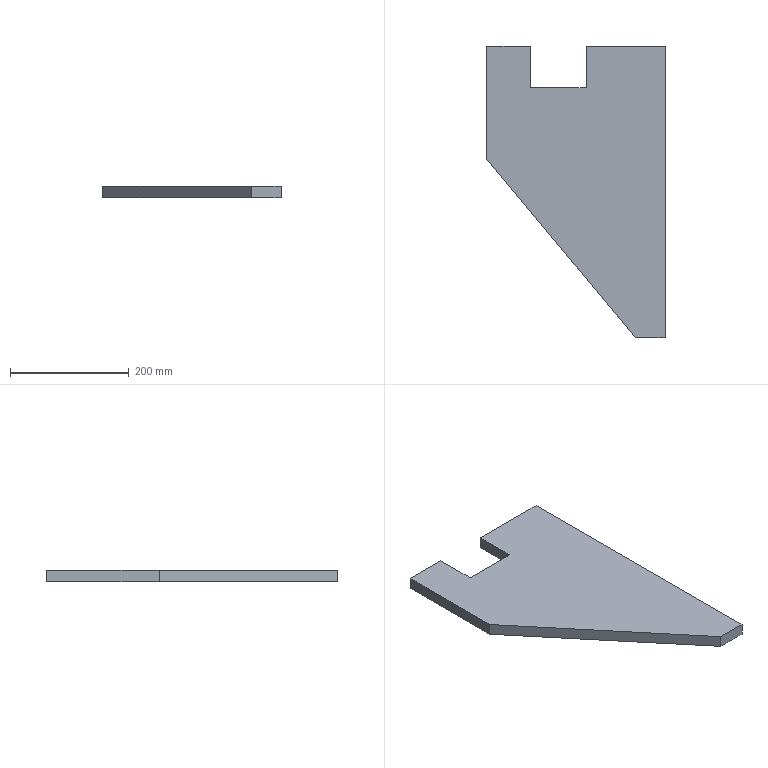Part | SolidWorks | features Extrusion 1 | 1 solid | 11 faces | box 300 x 490 x 20 mm | volume 2058400 mm3 | plane 11
STEP:
#1=CARTESIAN_POINT('',(0.,0.,0.));
#2=VERTEX_POINT('',#1);
#3=CARTESIAN_POINT('',(-133.,0.,0.));
#4=VERTEX_POINT('',#3);
#5=CARTESIAN_POINT('',(-133.,0.,0.));
#6=DIRECTION('',(-1.,0.,0.));
#7=VECTOR('',#6,1000.);
#8=LINE('',#5,#7);
#9=EDGE_CURVE('',#2,#4,#8,.T.);
#10=ORIENTED_EDGE('',*,*,#9,.T.);
#11=CARTESIAN_POINT('',(-133.,0.,20.));
#12=VERTEX_POINT('',#11);
#13=CARTESIAN_POINT('',(-133.,0.,20.));
#14=DIRECTION('',(0.,0.,-1.));
#15=VECTOR('',#14,1000.);
#16=LINE('',#13,#15);
#17=EDGE_CURVE('',#12,#4,#16,.T.);
#18=ORIENTED_EDGE('',*,*,#17,.F.);
#19=CARTESIAN_POINT('',(0.,0.,20.));
#20=VERTEX_POINT('',#19);
#21=CARTESIAN_POINT('',(-133.,0.,20.));
#22=DIRECTION('',(-1.,0.,0.));
#23=VECTOR('',#22,1000.);
#24=LINE('',#21,#23);
#25=EDGE_CURVE('',#20,#12,#24,.T.);
#26=ORIENTED_EDGE('',*,*,#25,.F.);
#27=CARTESIAN_POINT('',(0.,0.,20.));
#28=DIRECTION('',(0.,0.,-1.));
#29=VECTOR('',#28,1000.);
#30=LINE('',#27,#29);
#31=EDGE_CURVE('',#20,#2,#30,.T.);
#32=ORIENTED_EDGE('',*,*,#31,.T.);
#33=EDGE_LOOP('',(#10,#18,#26,#32));
#34=FACE_OUTER_BOUND('',#33,.T.);
#35=CARTESIAN_POINT('',(-133.,0.,20.));
#36=DIRECTION('',(0.,-1.,0.));
#37=DIRECTION('',(0.,0.,-1.));
#38=AXIS2_PLACEMENT_3D('',#35,#36,#37);
#39=PLANE('',#38);
#40=ADVANCED_FACE('',(#34),#39,.F.);
#41=CARTESIAN_POINT('',(-133.,-70.,0.));
#42=VERTEX_POINT('',#41);
#43=CARTESIAN_POINT('',(-133.,-70.,0.));
#44=DIRECTION('',(0.,-1.,0.));
#45=VECTOR('',#44,1000.);
#46=LINE('',#43,#45);
#47=EDGE_CURVE('',#4,#42,#46,.T.);
#48=ORIENTED_EDGE('',*,*,#47,.T.);
#49=CARTESIAN_POINT('',(-133.,-70.,20.));
#50=VERTEX_POINT('',#49);
#51=CARTESIAN_POINT('',(-133.,-70.,20.));
#52=DIRECTION('',(0.,0.,-1.));
#53=VECTOR('',#52,1000.);
#54=LINE('',#51,#53);
#55=EDGE_CURVE('',#50,#42,#54,.T.);
#56=ORIENTED_EDGE('',*,*,#55,.F.);
#57=CARTESIAN_POINT('',(-133.,-70.,20.));
#58=DIRECTION('',(0.,-1.,0.));
#59=VECTOR('',#58,1000.);
#60=LINE('',#57,#59);
#61=EDGE_CURVE('',#12,#50,#60,.T.);
#62=ORIENTED_EDGE('',*,*,#61,.F.);
#63=ORIENTED_EDGE('',*,*,#17,.T.);
#64=EDGE_LOOP('',(#48,#56,#62,#63));
#65=FACE_OUTER_BOUND('',#64,.T.);
#66=CARTESIAN_POINT('',(-133.,-70.,20.));
#67=DIRECTION('',(1.,0.,0.));
#68=DIRECTION('',(0.,0.,-1.));
#69=AXIS2_PLACEMENT_3D('',#66,#67,#68);
#70=PLANE('',#69);
#71=ADVANCED_FACE('',(#65),#70,.F.);
#72=CARTESIAN_POINT('',(-227.,-70.,0.));
#73=VERTEX_POINT('',#72);
#74=CARTESIAN_POINT('',(-227.,-70.,0.));
#75=DIRECTION('',(-1.,0.,0.));
#76=VECTOR('',#75,1000.);
#77=LINE('',#74,#76);
#78=EDGE_CURVE('',#42,#73,#77,.T.);
#79=ORIENTED_EDGE('',*,*,#78,.T.);
#80=CARTESIAN_POINT('',(-227.,-70.,20.));
#81=VERTEX_POINT('',#80);
#82=CARTESIAN_POINT('',(-227.,-70.,20.));
#83=DIRECTION('',(0.,0.,-1.));
#84=VECTOR('',#83,1000.);
#85=LINE('',#82,#84);
#86=EDGE_CURVE('',#81,#73,#85,.T.);
#87=ORIENTED_EDGE('',*,*,#86,.F.);
#88=CARTESIAN_POINT('',(-227.,-70.,20.));
#89=DIRECTION('',(-1.,0.,0.));
#90=VECTOR('',#89,1000.);
#91=LINE('',#88,#90);
#92=EDGE_CURVE('',#50,#81,#91,.T.);
#93=ORIENTED_EDGE('',*,*,#92,.F.);
#94=ORIENTED_EDGE('',*,*,#55,.T.);
#95=EDGE_LOOP('',(#79,#87,#93,#94));
#96=FACE_OUTER_BOUND('',#95,.T.);
#97=CARTESIAN_POINT('',(-227.,-70.,20.));
#98=DIRECTION('',(0.,-1.,0.));
#99=DIRECTION('',(0.,0.,-1.));
#100=AXIS2_PLACEMENT_3D('',#97,#98,#99);
#101=PLANE('',#100);
#102=ADVANCED_FACE('',(#96),#101,.F.);
#103=CARTESIAN_POINT('',(-227.,0.,0.));
#104=VERTEX_POINT('',#103);
#105=CARTESIAN_POINT('',(-227.,0.,0.));
#106=DIRECTION('',(0.,1.,0.));
#107=VECTOR('',#106,1000.);
#108=LINE('',#105,#107);
#109=EDGE_CURVE('',#73,#104,#108,.T.);
#110=ORIENTED_EDGE('',*,*,#109,.T.);
#111=CARTESIAN_POINT('',(-227.,0.,20.));
#112=VERTEX_POINT('',#111);
#113=CARTESIAN_POINT('',(-227.,0.,20.));
#114=DIRECTION('',(0.,0.,-1.));
#115=VECTOR('',#114,1000.);
#116=LINE('',#113,#115);
#117=EDGE_CURVE('',#112,#104,#116,.T.);
#118=ORIENTED_EDGE('',*,*,#117,.F.);
#119=CARTESIAN_POINT('',(-227.,0.,20.));
#120=DIRECTION('',(0.,1.,0.));
#121=VECTOR('',#120,1000.);
#122=LINE('',#119,#121);
#123=EDGE_CURVE('',#81,#112,#122,.T.);
#124=ORIENTED_EDGE('',*,*,#123,.F.);
#125=ORIENTED_EDGE('',*,*,#86,.T.);
#126=EDGE_LOOP('',(#110,#118,#124,#125));
#127=FACE_OUTER_BOUND('',#126,.T.);
#128=CARTESIAN_POINT('',(-227.,0.,20.));
#129=DIRECTION('',(-1.,0.,0.));
#130=DIRECTION('',(0.,0.,1.));
#131=AXIS2_PLACEMENT_3D('',#128,#129,#130);
#132=PLANE('',#131);
#133=ADVANCED_FACE('',(#127),#132,.F.);
#134=CARTESIAN_POINT('',(-300.,0.,0.));
#135=VERTEX_POINT('',#134);
#136=CARTESIAN_POINT('',(-300.,0.,0.));
#137=DIRECTION('',(-1.,0.,0.));
#138=VECTOR('',#137,1000.);
#139=LINE('',#136,#138);
#140=EDGE_CURVE('',#104,#135,#139,.T.);
#141=ORIENTED_EDGE('',*,*,#140,.T.);
#142=CARTESIAN_POINT('',(-300.,0.,20.));
#143=VERTEX_POINT('',#142);
#144=CARTESIAN_POINT('',(-300.,0.,20.));
#145=DIRECTION('',(0.,0.,-1.));
#146=VECTOR('',#145,1000.);
#147=LINE('',#144,#146);
#148=EDGE_CURVE('',#143,#135,#147,.T.);
#149=ORIENTED_EDGE('',*,*,#148,.F.);
#150=CARTESIAN_POINT('',(-300.,0.,20.));
#151=DIRECTION('',(-1.,0.,0.));
#152=VECTOR('',#151,1000.);
#153=LINE('',#150,#152);
#154=EDGE_CURVE('',#112,#143,#153,.T.);
#155=ORIENTED_EDGE('',*,*,#154,.F.);
#156=ORIENTED_EDGE('',*,*,#117,.T.);
#157=EDGE_LOOP('',(#141,#149,#155,#156));
#158=FACE_OUTER_BOUND('',#157,.T.);
#159=CARTESIAN_POINT('',(-300.,0.,20.));
#160=DIRECTION('',(0.,-1.,0.));
#161=DIRECTION('',(0.,0.,-1.));
#162=AXIS2_PLACEMENT_3D('',#159,#160,#161);
#163=PLANE('',#162);
#164=ADVANCED_FACE('',(#158),#163,.F.);
#165=CARTESIAN_POINT('',(-300.,-190.,0.));
#166=VERTEX_POINT('',#165);
#167=CARTESIAN_POINT('',(-300.,-190.,0.));
#168=DIRECTION('',(0.,-1.,0.));
#169=VECTOR('',#168,1000.);
#170=LINE('',#167,#169);
#171=EDGE_CURVE('',#135,#166,#170,.T.);
#172=ORIENTED_EDGE('',*,*,#171,.T.);
#173=CARTESIAN_POINT('',(-300.,-190.,20.));
#174=VERTEX_POINT('',#173);
#175=CARTESIAN_POINT('',(-300.,-190.,20.));
#176=DIRECTION('',(0.,0.,-1.));
#177=VECTOR('',#176,1000.);
#178=LINE('',#175,#177);
#179=EDGE_CURVE('',#174,#166,#178,.T.);
#180=ORIENTED_EDGE('',*,*,#179,.F.);
#181=CARTESIAN_POINT('',(-300.,-190.,20.));
#182=DIRECTION('',(0.,-1.,0.));
#183=VECTOR('',#182,1000.);
#184=LINE('',#181,#183);
#185=EDGE_CURVE('',#143,#174,#184,.T.);
#186=ORIENTED_EDGE('',*,*,#185,.F.);
#187=ORIENTED_EDGE('',*,*,#148,.T.);
#188=EDGE_LOOP('',(#172,#180,#186,#187));
#189=FACE_OUTER_BOUND('',#188,.T.);
#190=CARTESIAN_POINT('',(-300.,-190.,20.));
#191=DIRECTION('',(1.,0.,0.));
#192=DIRECTION('',(0.,0.,-1.));
#193=AXIS2_PLACEMENT_3D('',#190,#191,#192);
#194=PLANE('',#193);
#195=ADVANCED_FACE('',(#189),#194,.F.);
#196=CARTESIAN_POINT('',(-50.,-490.,0.));
#197=VERTEX_POINT('',#196);
#198=CARTESIAN_POINT('',(-50.,-490.,0.));
#199=DIRECTION('',(0.6402,-0.7682,0.));
#200=VECTOR('',#199,1000.);
#201=LINE('',#198,#200);
#202=EDGE_CURVE('',#166,#197,#201,.T.);
#203=ORIENTED_EDGE('',*,*,#202,.T.);
#204=CARTESIAN_POINT('',(-50.,-490.,20.));
#205=VERTEX_POINT('',#204);
#206=CARTESIAN_POINT('',(-50.,-490.,20.));
#207=DIRECTION('',(0.,0.,-1.));
#208=VECTOR('',#207,1000.);
#209=LINE('',#206,#208);
#210=EDGE_CURVE('',#205,#197,#209,.T.);
#211=ORIENTED_EDGE('',*,*,#210,.F.);
#212=CARTESIAN_POINT('',(-50.,-490.,20.));
#213=DIRECTION('',(0.6402,-0.7682,0.));
#214=VECTOR('',#213,1000.);
#215=LINE('',#212,#214);
#216=EDGE_CURVE('',#174,#205,#215,.T.);
#217=ORIENTED_EDGE('',*,*,#216,.F.);
#218=ORIENTED_EDGE('',*,*,#179,.T.);
#219=EDGE_LOOP('',(#203,#211,#217,#218));
#220=FACE_OUTER_BOUND('',#219,.T.);
#221=CARTESIAN_POINT('',(-50.,-490.,20.));
#222=DIRECTION('',(0.7682,0.6402,0.));
#223=DIRECTION('',(-0.6402,0.7682,0.));
#224=AXIS2_PLACEMENT_3D('',#221,#222,#223);
#225=PLANE('',#224);
#226=ADVANCED_FACE('',(#220),#225,.F.);
#227=CARTESIAN_POINT('',(0.,-490.,0.));
#228=VERTEX_POINT('',#227);
#229=CARTESIAN_POINT('',(0.,-490.,0.));
#230=DIRECTION('',(1.,0.,0.));
#231=VECTOR('',#230,1000.);
#232=LINE('',#229,#231);
#233=EDGE_CURVE('',#197,#228,#232,.T.);
#234=ORIENTED_EDGE('',*,*,#233,.T.);
#235=CARTESIAN_POINT('',(0.,-490.,20.));
#236=VERTEX_POINT('',#235);
#237=CARTESIAN_POINT('',(0.,-490.,20.));
#238=DIRECTION('',(0.,0.,-1.));
#239=VECTOR('',#238,1000.);
#240=LINE('',#237,#239);
#241=EDGE_CURVE('',#236,#228,#240,.T.);
#242=ORIENTED_EDGE('',*,*,#241,.F.);
#243=CARTESIAN_POINT('',(0.,-490.,20.));
#244=DIRECTION('',(1.,0.,0.));
#245=VECTOR('',#244,1000.);
#246=LINE('',#243,#245);
#247=EDGE_CURVE('',#205,#236,#246,.T.);
#248=ORIENTED_EDGE('',*,*,#247,.F.);
#249=ORIENTED_EDGE('',*,*,#210,.T.);
#250=EDGE_LOOP('',(#234,#242,#248,#249));
#251=FACE_OUTER_BOUND('',#250,.T.);
#252=CARTESIAN_POINT('',(0.,-490.,20.));
#253=DIRECTION('',(0.,1.,0.));
#254=DIRECTION('',(0.,0.,1.));
#255=AXIS2_PLACEMENT_3D('',#252,#253,#254);
#256=PLANE('',#255);
#257=ADVANCED_FACE('',(#251),#256,.F.);
#258=CARTESIAN_POINT('',(0.,0.,0.));
#259=DIRECTION('',(0.,1.,0.));
#260=VECTOR('',#259,1000.);
#261=LINE('',#258,#260);
#262=EDGE_CURVE('',#228,#2,#261,.T.);
#263=ORIENTED_EDGE('',*,*,#262,.T.);
#264=ORIENTED_EDGE('',*,*,#31,.F.);
#265=CARTESIAN_POINT('',(0.,0.,20.));
#266=DIRECTION('',(0.,1.,0.));
#267=VECTOR('',#266,1000.);
#268=LINE('',#265,#267);
#269=EDGE_CURVE('',#236,#20,#268,.T.);
#270=ORIENTED_EDGE('',*,*,#269,.F.);
#271=ORIENTED_EDGE('',*,*,#241,.T.);
#272=EDGE_LOOP('',(#263,#264,#270,#271));
#273=FACE_OUTER_BOUND('',#272,.T.);
#274=CARTESIAN_POINT('',(0.,0.,20.));
#275=DIRECTION('',(-1.,0.,0.));
#276=DIRECTION('',(0.,-1.,0.));
#277=AXIS2_PLACEMENT_3D('',#274,#275,#276);
#278=PLANE('',#277);
#279=ADVANCED_FACE('',(#273),#278,.F.);
#280=ORIENTED_EDGE('',*,*,#25,.T.);
#281=ORIENTED_EDGE('',*,*,#61,.T.);
#282=ORIENTED_EDGE('',*,*,#92,.T.);
#283=ORIENTED_EDGE('',*,*,#123,.T.);
#284=ORIENTED_EDGE('',*,*,#154,.T.);
#285=ORIENTED_EDGE('',*,*,#185,.T.);
#286=ORIENTED_EDGE('',*,*,#216,.T.);
#287=ORIENTED_EDGE('',*,*,#247,.T.);
#288=ORIENTED_EDGE('',*,*,#269,.T.);
#289=EDGE_LOOP('',(#280,#281,#282,#283,#284,#285,#286,#287,#288));
#290=FACE_OUTER_BOUND('',#289,.T.);
#291=CARTESIAN_POINT('',(0.,0.,20.));
#292=DIRECTION('',(0.,0.,-1.));
#293=DIRECTION('',(-1.,0.,0.));
#294=AXIS2_PLACEMENT_3D('',#291,#292,#293);
#295=PLANE('',#294);
#296=ADVANCED_FACE('',(#290),#295,.F.);
#297=ORIENTED_EDGE('',*,*,#9,.F.);
#298=ORIENTED_EDGE('',*,*,#262,.F.);
#299=ORIENTED_EDGE('',*,*,#233,.F.);
#300=ORIENTED_EDGE('',*,*,#202,.F.);
#301=ORIENTED_EDGE('',*,*,#171,.F.);
#302=ORIENTED_EDGE('',*,*,#140,.F.);
#303=ORIENTED_EDGE('',*,*,#109,.F.);
#304=ORIENTED_EDGE('',*,*,#78,.F.);
#305=ORIENTED_EDGE('',*,*,#47,.F.);
#306=EDGE_LOOP('',(#297,#298,#299,#300,#301,#302,#303,#304,#305));
#307=FACE_OUTER_BOUND('',#306,.T.);
#308=CARTESIAN_POINT('',(0.,0.,0.));
#309=DIRECTION('',(0.,0.,-1.));
#310=DIRECTION('',(-1.,0.,0.));
#311=AXIS2_PLACEMENT_3D('',#308,#309,#310);
#312=PLANE('',#311);
#313=ADVANCED_FACE('',(#307),#312,.T.);
#314=CLOSED_SHELL('',(#40,#71,#102,#133,#164,#195,#226,#257,#279,#296,#313));
#315=MANIFOLD_SOLID_BREP('',#314);
#316=CARTESIAN_POINT('',(0.,0.,0.));
#317=DIRECTION('',(0.,0.,1.));
#318=DIRECTION('',(1.,0.,0.));
#319=AXIS2_PLACEMENT_3D('',#316,#317,#318);
#320=(LENGTH_UNIT()NAMED_UNIT(*)SI_UNIT(.MILLI.,.METRE.));
#321=UNCERTAINTY_MEASURE_WITH_UNIT(LENGTH_MEASURE(0.00001),#320,'','');
#322=(NAMED_UNIT(*)PLANE_ANGLE_UNIT()SI_UNIT($,.RADIAN.));
#323=(NAMED_UNIT(*)SI_UNIT($,.STERADIAN.)SOLID_ANGLE_UNIT());
#324=(GEOMETRIC_REPRESENTATION_CONTEXT(3)GLOBAL_UNCERTAINTY_ASSIGNED_CONTEXT((#321))GLOBAL_UNIT_ASSIGNED_CONTEXT((#320,#322,#323))REPRESENTATION_CONTEXT('',''));
#325=ADVANCED_BREP_SHAPE_REPRESENTATION('',(#315,#319),#324);